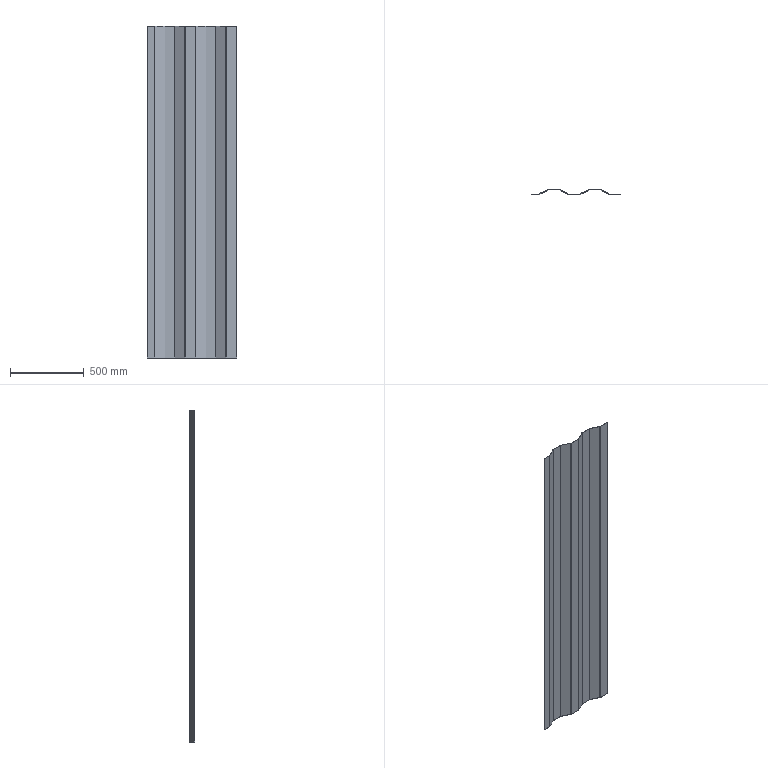Part | STEP file | 750078177 | 1 solid | 38 faces | box 606 x 36 x 2253 mm | volume 2873440 mm3 | plane 22 | cylinder 16 | commonest cylinder face diameters 6 x8 10 x8
STEP:
#1=CARTESIAN_POINT('',(116.472,35.472,0.));
#2=VERTEX_POINT('',#1);
#3=CARTESIAN_POINT('',(50.161,2.317,0.));
#4=VERTEX_POINT('',#3);
#5=CARTESIAN_POINT('',(117.106,35.789,0.));
#6=DIRECTION('',(-0.8944,-0.4472,0.));
#7=VECTOR('',#6,1000.);
#8=LINE('',#5,#7);
#9=EDGE_CURVE('',#2,#4,#8,.T.);
#10=ORIENTED_EDGE('',*,*,#9,.T.);
#11=CARTESIAN_POINT('',(50.161,2.317,2252.5));
#12=VERTEX_POINT('',#11);
#13=CARTESIAN_POINT('',(50.161,2.317,0.));
#14=DIRECTION('',(0.,0.,1.));
#15=VECTOR('',#14,1000.);
#16=LINE('',#13,#15);
#17=EDGE_CURVE('',#4,#12,#16,.T.);
#18=ORIENTED_EDGE('',*,*,#17,.T.);
#19=CARTESIAN_POINT('',(116.472,35.472,2252.5));
#20=VERTEX_POINT('',#19);
#21=CARTESIAN_POINT('',(117.106,35.789,2252.5));
#22=DIRECTION('',(0.8944,0.4472,0.));
#23=VECTOR('',#22,1000.);
#24=LINE('',#21,#23);
#25=EDGE_CURVE('',#12,#20,#24,.T.);
#26=ORIENTED_EDGE('',*,*,#25,.T.);
#27=CARTESIAN_POINT('',(116.472,35.472,0.));
#28=DIRECTION('',(0.,0.,-1.));
#29=VECTOR('',#28,1000.);
#30=LINE('',#27,#29);
#31=EDGE_CURVE('',#20,#2,#30,.T.);
#32=ORIENTED_EDGE('',*,*,#31,.T.);
#33=EDGE_LOOP('',(#10,#18,#26,#32));
#34=FACE_OUTER_BOUND('',#33,.T.);
#35=CARTESIAN_POINT('',(117.106,35.789,0.));
#36=DIRECTION('',(-0.4472,0.8944,0.));
#37=DIRECTION('',(-0.8944,-0.4472,0.));
#38=AXIS2_PLACEMENT_3D('',#35,#36,#37);
#39=PLANE('',#38);
#40=ADVANCED_FACE('',(#34),#39,.T.);
#41=ORIENTED_EDGE('',*,*,#17,.F.);
#42=CARTESIAN_POINT('',(48.82,2.,0.));
#43=VERTEX_POINT('',#42);
#44=CARTESIAN_POINT('',(48.82,5.,0.));
#45=DIRECTION('',(0.,0.,1.));
#46=DIRECTION('',(1.,0.,0.));
#47=AXIS2_PLACEMENT_3D('',#44,#45,#46);
#48=CIRCLE('',#47,3.);
#49=EDGE_CURVE('',#43,#4,#48,.T.);
#50=ORIENTED_EDGE('',*,*,#49,.F.);
#51=CARTESIAN_POINT('',(48.82,2.,2252.5));
#52=VERTEX_POINT('',#51);
#53=CARTESIAN_POINT('',(48.82,2.,0.));
#54=DIRECTION('',(0.,0.,-1.));
#55=VECTOR('',#54,1000.);
#56=LINE('',#53,#55);
#57=EDGE_CURVE('',#52,#43,#56,.T.);
#58=ORIENTED_EDGE('',*,*,#57,.F.);
#59=CARTESIAN_POINT('',(48.82,5.,2252.5));
#60=DIRECTION('',(0.,0.,-1.));
#61=DIRECTION('',(1.,0.,0.));
#62=AXIS2_PLACEMENT_3D('',#59,#60,#61);
#63=CIRCLE('',#62,3.);
#64=EDGE_CURVE('',#12,#52,#63,.T.);
#65=ORIENTED_EDGE('',*,*,#64,.F.);
#66=EDGE_LOOP('',(#41,#50,#58,#65));
#67=FACE_OUTER_BOUND('',#66,.T.);
#68=CARTESIAN_POINT('',(48.82,5.,0.));
#69=DIRECTION('',(0.,0.,1.));
#70=DIRECTION('',(1.,0.,0.));
#71=AXIS2_PLACEMENT_3D('',#68,#69,#70);
#72=CYLINDRICAL_SURFACE('',#71,3.);
#73=ADVANCED_FACE('',(#67),#72,.F.);
#74=CARTESIAN_POINT('',(535.18,2.,0.));
#75=VERTEX_POINT('',#74);
#76=CARTESIAN_POINT('',(606.,2.,0.));
#77=VERTEX_POINT('',#76);
#78=CARTESIAN_POINT('',(606.,2.,0.));
#79=DIRECTION('',(1.,0.,0.));
#80=VECTOR('',#79,1000.);
#81=LINE('',#78,#80);
#82=EDGE_CURVE('',#75,#77,#81,.T.);
#83=ORIENTED_EDGE('',*,*,#82,.T.);
#84=CARTESIAN_POINT('',(606.,0.,0.));
#85=VERTEX_POINT('',#84);
#86=CARTESIAN_POINT('',(606.,0.,0.));
#87=DIRECTION('',(0.,-1.,0.));
#88=VECTOR('',#87,1000.);
#89=LINE('',#86,#88);
#90=EDGE_CURVE('',#77,#85,#89,.T.);
#91=ORIENTED_EDGE('',*,*,#90,.T.);
#92=CARTESIAN_POINT('',(535.18,0.,0.));
#93=VERTEX_POINT('',#92);
#94=CARTESIAN_POINT('',(606.,0.,0.));
#95=DIRECTION('',(-1.,0.,0.));
#96=VECTOR('',#95,1000.);
#97=LINE('',#94,#96);
#98=EDGE_CURVE('',#85,#93,#97,.T.);
#99=ORIENTED_EDGE('',*,*,#98,.T.);
#100=CARTESIAN_POINT('',(532.944,0.5279,0.));
#101=VERTEX_POINT('',#100);
#102=CARTESIAN_POINT('',(535.18,5.,0.));
#103=DIRECTION('',(0.,0.,-1.));
#104=DIRECTION('',(1.,0.,0.));
#105=AXIS2_PLACEMENT_3D('',#102,#103,#104);
#106=CIRCLE('',#105,5.);
#107=EDGE_CURVE('',#93,#101,#106,.T.);
#108=ORIENTED_EDGE('',*,*,#107,.T.);
#109=CARTESIAN_POINT('',(466.633,33.683,0.));
#110=VERTEX_POINT('',#109);
#111=CARTESIAN_POINT('',(532.944,0.5279,0.));
#112=DIRECTION('',(-0.8944,0.4472,0.));
#113=VECTOR('',#112,1000.);
#114=LINE('',#111,#113);
#115=EDGE_CURVE('',#101,#110,#114,.T.);
#116=ORIENTED_EDGE('',*,*,#115,.T.);
#117=CARTESIAN_POINT('',(465.292,34.,0.));
#118=VERTEX_POINT('',#117);
#119=CARTESIAN_POINT('',(465.292,31.,0.));
#120=DIRECTION('',(0.,0.,1.));
#121=DIRECTION('',(1.,0.,0.));
#122=AXIS2_PLACEMENT_3D('',#119,#120,#121);
#123=CIRCLE('',#122,3.);
#124=EDGE_CURVE('',#110,#118,#123,.T.);
#125=ORIENTED_EDGE('',*,*,#124,.T.);
#126=CARTESIAN_POINT('',(396.708,34.,0.));
#127=VERTEX_POINT('',#126);
#128=CARTESIAN_POINT('',(606.,34.,0.));
#129=DIRECTION('',(-1.,0.,0.));
#130=VECTOR('',#129,1000.);
#131=LINE('',#128,#130);
#132=EDGE_CURVE('',#118,#127,#131,.T.);
#133=ORIENTED_EDGE('',*,*,#132,.T.);
#134=CARTESIAN_POINT('',(395.367,33.683,0.));
#135=VERTEX_POINT('',#134);
#136=CARTESIAN_POINT('',(396.708,31.,0.));
#137=DIRECTION('',(0.,0.,1.));
#138=DIRECTION('',(1.,0.,0.));
#139=AXIS2_PLACEMENT_3D('',#136,#137,#138);
#140=CIRCLE('',#139,3.);
#141=EDGE_CURVE('',#127,#135,#140,.T.);
#142=ORIENTED_EDGE('',*,*,#141,.T.);
#143=CARTESIAN_POINT('',(329.056,0.5279,0.));
#144=VERTEX_POINT('',#143);
#145=CARTESIAN_POINT('',(395.367,33.683,0.));
#146=DIRECTION('',(-0.8944,-0.4472,0.));
#147=VECTOR('',#146,1000.);
#148=LINE('',#145,#147);
#149=EDGE_CURVE('',#135,#144,#148,.T.);
#150=ORIENTED_EDGE('',*,*,#149,.T.);
#151=CARTESIAN_POINT('',(326.82,0.,0.));
#152=VERTEX_POINT('',#151);
#153=CARTESIAN_POINT('',(326.82,5.,0.));
#154=DIRECTION('',(0.,0.,-1.));
#155=DIRECTION('',(1.,0.,0.));
#156=AXIS2_PLACEMENT_3D('',#153,#154,#155);
#157=CIRCLE('',#156,5.);
#158=EDGE_CURVE('',#144,#152,#157,.T.);
#159=ORIENTED_EDGE('',*,*,#158,.T.);
#160=CARTESIAN_POINT('',(257.18,0.,0.));
#161=VERTEX_POINT('',#160);
#162=CARTESIAN_POINT('',(606.,0.,0.));
#163=DIRECTION('',(-1.,0.,0.));
#164=VECTOR('',#163,1000.);
#165=LINE('',#162,#164);
#166=EDGE_CURVE('',#152,#161,#165,.T.);
#167=ORIENTED_EDGE('',*,*,#166,.T.);
#168=CARTESIAN_POINT('',(254.944,0.5279,0.));
#169=VERTEX_POINT('',#168);
#170=CARTESIAN_POINT('',(257.18,5.,0.));
#171=DIRECTION('',(0.,0.,-1.));
#172=DIRECTION('',(1.,0.,0.));
#173=AXIS2_PLACEMENT_3D('',#170,#171,#172);
#174=CIRCLE('',#173,5.);
#175=EDGE_CURVE('',#161,#169,#174,.T.);
#176=ORIENTED_EDGE('',*,*,#175,.T.);
#177=CARTESIAN_POINT('',(188.633,33.683,0.));
#178=VERTEX_POINT('',#177);
#179=CARTESIAN_POINT('',(254.944,0.5279,0.));
#180=DIRECTION('',(-0.8944,0.4472,0.));
#181=VECTOR('',#180,1000.);
#182=LINE('',#179,#181);
#183=EDGE_CURVE('',#169,#178,#182,.T.);
#184=ORIENTED_EDGE('',*,*,#183,.T.);
#185=CARTESIAN_POINT('',(187.292,34.,0.));
#186=VERTEX_POINT('',#185);
#187=CARTESIAN_POINT('',(187.292,31.,0.));
#188=DIRECTION('',(0.,0.,1.));
#189=DIRECTION('',(1.,0.,0.));
#190=AXIS2_PLACEMENT_3D('',#187,#188,#189);
#191=CIRCLE('',#190,3.);
#192=EDGE_CURVE('',#178,#186,#191,.T.);
#193=ORIENTED_EDGE('',*,*,#192,.T.);
#194=CARTESIAN_POINT('',(118.708,34.,0.));
#195=VERTEX_POINT('',#194);
#196=CARTESIAN_POINT('',(606.,34.,0.));
#197=DIRECTION('',(-1.,0.,0.));
#198=VECTOR('',#197,1000.);
#199=LINE('',#196,#198);
#200=EDGE_CURVE('',#186,#195,#199,.T.);
#201=ORIENTED_EDGE('',*,*,#200,.T.);
#202=CARTESIAN_POINT('',(117.367,33.683,0.));
#203=VERTEX_POINT('',#202);
#204=CARTESIAN_POINT('',(118.708,31.,0.));
#205=DIRECTION('',(0.,0.,1.));
#206=DIRECTION('',(1.,0.,0.));
#207=AXIS2_PLACEMENT_3D('',#204,#205,#206);
#208=CIRCLE('',#207,3.);
#209=EDGE_CURVE('',#195,#203,#208,.T.);
#210=ORIENTED_EDGE('',*,*,#209,.T.);
#211=CARTESIAN_POINT('',(51.056,0.5279,0.));
#212=VERTEX_POINT('',#211);
#213=CARTESIAN_POINT('',(117.367,33.683,0.));
#214=DIRECTION('',(-0.8944,-0.4472,0.));
#215=VECTOR('',#214,1000.);
#216=LINE('',#213,#215);
#217=EDGE_CURVE('',#203,#212,#216,.T.);
#218=ORIENTED_EDGE('',*,*,#217,.T.);
#219=CARTESIAN_POINT('',(48.82,0.,0.));
#220=VERTEX_POINT('',#219);
#221=CARTESIAN_POINT('',(48.82,5.,0.));
#222=DIRECTION('',(0.,0.,-1.));
#223=DIRECTION('',(1.,0.,0.));
#224=AXIS2_PLACEMENT_3D('',#221,#222,#223);
#225=CIRCLE('',#224,5.);
#226=EDGE_CURVE('',#212,#220,#225,.T.);
#227=ORIENTED_EDGE('',*,*,#226,.T.);
#228=CARTESIAN_POINT('',(0.,0.,0.));
#229=VERTEX_POINT('',#228);
#230=CARTESIAN_POINT('',(606.,0.,0.));
#231=DIRECTION('',(-1.,0.,0.));
#232=VECTOR('',#231,1000.);
#233=LINE('',#230,#232);
#234=EDGE_CURVE('',#220,#229,#233,.T.);
#235=ORIENTED_EDGE('',*,*,#234,.T.);
#236=CARTESIAN_POINT('',(0.,2.,0.));
#237=VERTEX_POINT('',#236);
#238=CARTESIAN_POINT('',(0.,0.,0.));
#239=DIRECTION('',(0.,1.,0.));
#240=VECTOR('',#239,1000.);
#241=LINE('',#238,#240);
#242=EDGE_CURVE('',#229,#237,#241,.T.);
#243=ORIENTED_EDGE('',*,*,#242,.T.);
#244=CARTESIAN_POINT('',(606.,2.,0.));
#245=DIRECTION('',(1.,0.,0.));
#246=VECTOR('',#245,1000.);
#247=LINE('',#244,#246);
#248=EDGE_CURVE('',#237,#43,#247,.T.);
#249=ORIENTED_EDGE('',*,*,#248,.T.);
#250=ORIENTED_EDGE('',*,*,#49,.T.);
#251=ORIENTED_EDGE('',*,*,#9,.F.);
#252=CARTESIAN_POINT('',(118.708,36.,0.));
#253=VERTEX_POINT('',#252);
#254=CARTESIAN_POINT('',(118.708,31.,0.));
#255=DIRECTION('',(0.,0.,-1.));
#256=DIRECTION('',(1.,0.,0.));
#257=AXIS2_PLACEMENT_3D('',#254,#255,#256);
#258=CIRCLE('',#257,5.);
#259=EDGE_CURVE('',#2,#253,#258,.T.);
#260=ORIENTED_EDGE('',*,*,#259,.T.);
#261=CARTESIAN_POINT('',(187.292,36.,0.));
#262=VERTEX_POINT('',#261);
#263=CARTESIAN_POINT('',(606.,36.,0.));
#264=DIRECTION('',(1.,0.,0.));
#265=VECTOR('',#264,1000.);
#266=LINE('',#263,#265);
#267=EDGE_CURVE('',#253,#262,#266,.T.);
#268=ORIENTED_EDGE('',*,*,#267,.T.);
#269=CARTESIAN_POINT('',(189.528,35.472,0.));
#270=VERTEX_POINT('',#269);
#271=CARTESIAN_POINT('',(187.292,31.,0.));
#272=DIRECTION('',(0.,0.,-1.));
#273=DIRECTION('',(1.,0.,0.));
#274=AXIS2_PLACEMENT_3D('',#271,#272,#273);
#275=CIRCLE('',#274,5.);
#276=EDGE_CURVE('',#262,#270,#275,.T.);
#277=ORIENTED_EDGE('',*,*,#276,.T.);
#278=CARTESIAN_POINT('',(255.839,2.317,0.));
#279=VERTEX_POINT('',#278);
#280=CARTESIAN_POINT('',(189.528,35.472,0.));
#281=DIRECTION('',(0.8944,-0.4472,0.));
#282=VECTOR('',#281,1000.);
#283=LINE('',#280,#282);
#284=EDGE_CURVE('',#270,#279,#283,.T.);
#285=ORIENTED_EDGE('',*,*,#284,.T.);
#286=CARTESIAN_POINT('',(257.18,2.,0.));
#287=VERTEX_POINT('',#286);
#288=CARTESIAN_POINT('',(257.18,5.,0.));
#289=DIRECTION('',(0.,0.,1.));
#290=DIRECTION('',(1.,0.,0.));
#291=AXIS2_PLACEMENT_3D('',#288,#289,#290);
#292=CIRCLE('',#291,3.);
#293=EDGE_CURVE('',#279,#287,#292,.T.);
#294=ORIENTED_EDGE('',*,*,#293,.T.);
#295=CARTESIAN_POINT('',(326.82,2.,0.));
#296=VERTEX_POINT('',#295);
#297=CARTESIAN_POINT('',(606.,2.,0.));
#298=DIRECTION('',(1.,0.,0.));
#299=VECTOR('',#298,1000.);
#300=LINE('',#297,#299);
#301=EDGE_CURVE('',#287,#296,#300,.T.);
#302=ORIENTED_EDGE('',*,*,#301,.T.);
#303=CARTESIAN_POINT('',(328.161,2.317,0.));
#304=VERTEX_POINT('',#303);
#305=CARTESIAN_POINT('',(326.82,5.,0.));
#306=DIRECTION('',(0.,0.,1.));
#307=DIRECTION('',(1.,0.,0.));
#308=AXIS2_PLACEMENT_3D('',#305,#306,#307);
#309=CIRCLE('',#308,3.);
#310=EDGE_CURVE('',#296,#304,#309,.T.);
#311=ORIENTED_EDGE('',*,*,#310,.T.);
#312=CARTESIAN_POINT('',(394.472,35.472,0.));
#313=VERTEX_POINT('',#312);
#314=CARTESIAN_POINT('',(328.161,2.317,0.));
#315=DIRECTION('',(0.8944,0.4472,0.));
#316=VECTOR('',#315,1000.);
#317=LINE('',#314,#316);
#318=EDGE_CURVE('',#304,#313,#317,.T.);
#319=ORIENTED_EDGE('',*,*,#318,.T.);
#320=CARTESIAN_POINT('',(396.708,36.,0.));
#321=VERTEX_POINT('',#320);
#322=CARTESIAN_POINT('',(396.708,31.,0.));
#323=DIRECTION('',(0.,0.,-1.));
#324=DIRECTION('',(1.,0.,0.));
#325=AXIS2_PLACEMENT_3D('',#322,#323,#324);
#326=CIRCLE('',#325,5.);
#327=EDGE_CURVE('',#313,#321,#326,.T.);
#328=ORIENTED_EDGE('',*,*,#327,.T.);
#329=CARTESIAN_POINT('',(465.292,36.,0.));
#330=VERTEX_POINT('',#329);
#331=CARTESIAN_POINT('',(606.,36.,0.));
#332=DIRECTION('',(1.,0.,0.));
#333=VECTOR('',#332,1000.);
#334=LINE('',#331,#333);
#335=EDGE_CURVE('',#321,#330,#334,.T.);
#336=ORIENTED_EDGE('',*,*,#335,.T.);
#337=CARTESIAN_POINT('',(467.528,35.472,0.));
#338=VERTEX_POINT('',#337);
#339=CARTESIAN_POINT('',(465.292,31.,0.));
#340=DIRECTION('',(0.,0.,-1.));
#341=DIRECTION('',(1.,0.,0.));
#342=AXIS2_PLACEMENT_3D('',#339,#340,#341);
#343=CIRCLE('',#342,5.);
#344=EDGE_CURVE('',#330,#338,#343,.T.);
#345=ORIENTED_EDGE('',*,*,#344,.T.);
#346=CARTESIAN_POINT('',(533.839,2.317,0.));
#347=VERTEX_POINT('',#346);
#348=CARTESIAN_POINT('',(467.528,35.472,0.));
#349=DIRECTION('',(0.8944,-0.4472,0.));
#350=VECTOR('',#349,1000.);
#351=LINE('',#348,#350);
#352=EDGE_CURVE('',#338,#347,#351,.T.);
#353=ORIENTED_EDGE('',*,*,#352,.T.);
#354=CARTESIAN_POINT('',(535.18,5.,0.));
#355=DIRECTION('',(0.,0.,1.));
#356=DIRECTION('',(1.,0.,0.));
#357=AXIS2_PLACEMENT_3D('',#354,#355,#356);
#358=CIRCLE('',#357,3.);
#359=EDGE_CURVE('',#347,#75,#358,.T.);
#360=ORIENTED_EDGE('',*,*,#359,.T.);
#361=EDGE_LOOP('',(#83,#91,#99,#108,#116,#125,#133,#142,#150,#159,#167,#176,#184,#193,#201,#210,#218,#227,#235,#243,#249,#250,#251,#260,#268,#277,#285,#294,#302,#311,#319,#328,#336,#345,#353,#360));
#362=FACE_OUTER_BOUND('',#361,.T.);
#363=CARTESIAN_POINT('',(606.,0.,0.));
#364=DIRECTION('',(0.,0.,-1.));
#365=DIRECTION('',(-1.,0.,0.));
#366=AXIS2_PLACEMENT_3D('',#363,#364,#365);
#367=PLANE('',#366);
#368=ADVANCED_FACE('',(#362),#367,.T.);
#369=ORIENTED_EDGE('',*,*,#259,.F.);
#370=ORIENTED_EDGE('',*,*,#31,.F.);
#371=CARTESIAN_POINT('',(118.708,36.,2252.5));
#372=VERTEX_POINT('',#371);
#373=CARTESIAN_POINT('',(118.708,31.,2252.5));
#374=DIRECTION('',(0.,0.,-1.));
#375=DIRECTION('',(1.,0.,0.));
#376=AXIS2_PLACEMENT_3D('',#373,#374,#375);
#377=CIRCLE('',#376,5.);
#378=EDGE_CURVE('',#20,#372,#377,.T.);
#379=ORIENTED_EDGE('',*,*,#378,.T.);
#380=CARTESIAN_POINT('',(118.708,36.,0.));
#381=DIRECTION('',(0.,0.,-1.));
#382=VECTOR('',#381,1000.);
#383=LINE('',#380,#382);
#384=EDGE_CURVE('',#372,#253,#383,.T.);
#385=ORIENTED_EDGE('',*,*,#384,.T.);
#386=EDGE_LOOP('',(#369,#370,#379,#385));
#387=FACE_OUTER_BOUND('',#386,.T.);
#388=CARTESIAN_POINT('',(118.708,31.,0.));
#389=DIRECTION('',(0.,0.,1.));
#390=DIRECTION('',(1.,0.,0.));
#391=AXIS2_PLACEMENT_3D('',#388,#389,#390);
#392=CYLINDRICAL_SURFACE('',#391,5.);
#393=ADVANCED_FACE('',(#387),#392,.T.);
#394=CARTESIAN_POINT('',(467.528,35.472,2252.5));
#395=VERTEX_POINT('',#394);
#396=CARTESIAN_POINT('',(533.839,2.317,2252.5));
#397=VERTEX_POINT('',#396);
#398=CARTESIAN_POINT('',(467.528,35.472,2252.5));
#399=DIRECTION('',(0.8944,-0.4472,0.));
#400=VECTOR('',#399,1000.);
#401=LINE('',#398,#400);
#402=EDGE_CURVE('',#395,#397,#401,.T.);
#403=ORIENTED_EDGE('',*,*,#402,.F.);
#404=CARTESIAN_POINT('',(465.292,36.,2252.5));
#405=VERTEX_POINT('',#404);
#406=CARTESIAN_POINT('',(465.292,31.,2252.5));
#407=DIRECTION('',(0.,0.,-1.));
#408=DIRECTION('',(1.,0.,0.));
#409=AXIS2_PLACEMENT_3D('',#406,#407,#408);
#410=CIRCLE('',#409,5.);
#411=EDGE_CURVE('',#405,#395,#410,.T.);
#412=ORIENTED_EDGE('',*,*,#411,.F.);
#413=CARTESIAN_POINT('',(396.708,36.,2252.5));
#414=VERTEX_POINT('',#413);
#415=CARTESIAN_POINT('',(535.18,36.,2252.5));
#416=DIRECTION('',(1.,0.,0.));
#417=VECTOR('',#416,1000.);
#418=LINE('',#415,#417);
#419=EDGE_CURVE('',#414,#405,#418,.T.);
#420=ORIENTED_EDGE('',*,*,#419,.F.);
#421=CARTESIAN_POINT('',(394.472,35.472,2252.5));
#422=VERTEX_POINT('',#421);
#423=CARTESIAN_POINT('',(396.708,31.,2252.5));
#424=DIRECTION('',(0.,0.,-1.));
#425=DIRECTION('',(1.,0.,0.));
#426=AXIS2_PLACEMENT_3D('',#423,#424,#425);
#427=CIRCLE('',#426,5.);
#428=EDGE_CURVE('',#422,#414,#427,.T.);
#429=ORIENTED_EDGE('',*,*,#428,.F.);
#430=CARTESIAN_POINT('',(328.161,2.317,2252.5));
#431=VERTEX_POINT('',#430);
#432=CARTESIAN_POINT('',(328.161,2.317,2252.5));
#433=DIRECTION('',(0.8944,0.4472,0.));
#434=VECTOR('',#433,1000.);
#435=LINE('',#432,#434);
#436=EDGE_CURVE('',#431,#422,#435,.T.);
#437=ORIENTED_EDGE('',*,*,#436,.F.);
#438=CARTESIAN_POINT('',(326.82,2.,2252.5));
#439=VERTEX_POINT('',#438);
#440=CARTESIAN_POINT('',(326.82,5.,2252.5));
#441=DIRECTION('',(0.,0.,-1.));
#442=DIRECTION('',(1.,0.,0.));
#443=AXIS2_PLACEMENT_3D('',#440,#441,#442);
#444=CIRCLE('',#443,3.);
#445=EDGE_CURVE('',#431,#439,#444,.T.);
#446=ORIENTED_EDGE('',*,*,#445,.T.);
#447=CARTESIAN_POINT('',(257.18,2.,2252.5));
#448=VERTEX_POINT('',#447);
#449=CARTESIAN_POINT('',(535.18,2.,2252.5));
#450=DIRECTION('',(1.,0.,0.));
#451=VECTOR('',#450,1000.);
#452=LINE('',#449,#451);
#453=EDGE_CURVE('',#448,#439,#452,.T.);
#454=ORIENTED_EDGE('',*,*,#453,.F.);
#455=CARTESIAN_POINT('',(255.839,2.317,2252.5));
#456=VERTEX_POINT('',#455);
#457=CARTESIAN_POINT('',(257.18,5.,2252.5));
#458=DIRECTION('',(0.,0.,-1.));
#459=DIRECTION('',(1.,0.,0.));
#460=AXIS2_PLACEMENT_3D('',#457,#458,#459);
#461=CIRCLE('',#460,3.);
#462=EDGE_CURVE('',#448,#456,#461,.T.);
#463=ORIENTED_EDGE('',*,*,#462,.T.);
#464=CARTESIAN_POINT('',(189.528,35.472,2252.5));
#465=VERTEX_POINT('',#464);
#466=CARTESIAN_POINT('',(189.528,35.472,2252.5));
#467=DIRECTION('',(0.8944,-0.4472,0.));
#468=VECTOR('',#467,1000.);
#469=LINE('',#466,#468);
#470=EDGE_CURVE('',#465,#456,#469,.T.);
#471=ORIENTED_EDGE('',*,*,#470,.F.);
#472=CARTESIAN_POINT('',(187.292,36.,2252.5));
#473=VERTEX_POINT('',#472);
#474=CARTESIAN_POINT('',(187.292,31.,2252.5));
#475=DIRECTION('',(0.,0.,-1.));
#476=DIRECTION('',(1.,0.,0.));
#477=AXIS2_PLACEMENT_3D('',#474,#475,#476);
#478=CIRCLE('',#477,5.);
#479=EDGE_CURVE('',#473,#465,#478,.T.);
#480=ORIENTED_EDGE('',*,*,#479,.F.);
#481=CARTESIAN_POINT('',(535.18,36.,2252.5));
#482=DIRECTION('',(1.,0.,0.));
#483=VECTOR('',#482,1000.);
#484=LINE('',#481,#483);
#485=EDGE_CURVE('',#372,#473,#484,.T.);
#486=ORIENTED_EDGE('',*,*,#485,.F.);
#487=ORIENTED_EDGE('',*,*,#378,.F.);
#488=ORIENTED_EDGE('',*,*,#25,.F.);
#489=ORIENTED_EDGE('',*,*,#64,.T.);
#490=CARTESIAN_POINT('',(0.,2.,2252.5));
#491=VERTEX_POINT('',#490);
#492=CARTESIAN_POINT('',(535.18,2.,2252.5));
#493=DIRECTION('',(1.,0.,0.));
#494=VECTOR('',#493,1000.);
#495=LINE('',#492,#494);
#496=EDGE_CURVE('',#491,#52,#495,.T.);
#497=ORIENTED_EDGE('',*,*,#496,.F.);
#498=CARTESIAN_POINT('',(0.,0.,2252.5));
#499=VERTEX_POINT('',#498);
#500=CARTESIAN_POINT('',(0.,5.,2252.5));
#501=DIRECTION('',(0.,1.,0.));
#502=VECTOR('',#501,1000.);
#503=LINE('',#500,#502);
#504=EDGE_CURVE('',#499,#491,#503,.T.);
#505=ORIENTED_EDGE('',*,*,#504,.F.);
#506=CARTESIAN_POINT('',(48.82,0.,2252.5));
#507=VERTEX_POINT('',#506);
#508=CARTESIAN_POINT('',(535.18,0.,2252.5));
#509=DIRECTION('',(-1.,0.,0.));
#510=VECTOR('',#509,1000.);
#511=LINE('',#508,#510);
#512=EDGE_CURVE('',#507,#499,#511,.T.);
#513=ORIENTED_EDGE('',*,*,#512,.F.);
#514=CARTESIAN_POINT('',(51.056,0.5279,2252.5));
#515=VERTEX_POINT('',#514);
#516=CARTESIAN_POINT('',(48.82,5.,2252.5));
#517=DIRECTION('',(0.,0.,-1.));
#518=DIRECTION('',(1.,0.,0.));
#519=AXIS2_PLACEMENT_3D('',#516,#517,#518);
#520=CIRCLE('',#519,5.);
#521=EDGE_CURVE('',#515,#507,#520,.T.);
#522=ORIENTED_EDGE('',*,*,#521,.F.);
#523=CARTESIAN_POINT('',(117.367,33.683,2252.5));
#524=VERTEX_POINT('',#523);
#525=CARTESIAN_POINT('',(117.367,33.683,2252.5));
#526=DIRECTION('',(-0.8944,-0.4472,0.));
#527=VECTOR('',#526,1000.);
#528=LINE('',#525,#527);
#529=EDGE_CURVE('',#524,#515,#528,.T.);
#530=ORIENTED_EDGE('',*,*,#529,.F.);
#531=CARTESIAN_POINT('',(118.708,34.,2252.5));
#532=VERTEX_POINT('',#531);
#533=CARTESIAN_POINT('',(118.708,31.,2252.5));
#534=DIRECTION('',(0.,0.,-1.));
#535=DIRECTION('',(1.,0.,0.));
#536=AXIS2_PLACEMENT_3D('',#533,#534,#535);
#537=CIRCLE('',#536,3.);
#538=EDGE_CURVE('',#524,#532,#537,.T.);
#539=ORIENTED_EDGE('',*,*,#538,.T.);
#540=CARTESIAN_POINT('',(187.292,34.,2252.5));
#541=VERTEX_POINT('',#540);
#542=CARTESIAN_POINT('',(535.18,34.,2252.5));
#543=DIRECTION('',(-1.,0.,0.));
#544=VECTOR('',#543,1000.);
#545=LINE('',#542,#544);
#546=EDGE_CURVE('',#541,#532,#545,.T.);
#547=ORIENTED_EDGE('',*,*,#546,.F.);
#548=CARTESIAN_POINT('',(188.633,33.683,2252.5));
#549=VERTEX_POINT('',#548);
#550=CARTESIAN_POINT('',(187.292,31.,2252.5));
#551=DIRECTION('',(0.,0.,-1.));
#552=DIRECTION('',(1.,0.,0.));
#553=AXIS2_PLACEMENT_3D('',#550,#551,#552);
#554=CIRCLE('',#553,3.);
#555=EDGE_CURVE('',#541,#549,#554,.T.);
#556=ORIENTED_EDGE('',*,*,#555,.T.);
#557=CARTESIAN_POINT('',(254.944,0.5279,2252.5));
#558=VERTEX_POINT('',#557);
#559=CARTESIAN_POINT('',(254.944,0.5279,2252.5));
#560=DIRECTION('',(-0.8944,0.4472,0.));
#561=VECTOR('',#560,1000.);
#562=LINE('',#559,#561);
#563=EDGE_CURVE('',#558,#549,#562,.T.);
#564=ORIENTED_EDGE('',*,*,#563,.F.);
#565=CARTESIAN_POINT('',(257.18,0.,2252.5));
#566=VERTEX_POINT('',#565);
#567=CARTESIAN_POINT('',(257.18,5.,2252.5));
#568=DIRECTION('',(0.,0.,-1.));
#569=DIRECTION('',(1.,0.,0.));
#570=AXIS2_PLACEMENT_3D('',#567,#568,#569);
#571=CIRCLE('',#570,5.);
#572=EDGE_CURVE('',#566,#558,#571,.T.);
#573=ORIENTED_EDGE('',*,*,#572,.F.);
#574=CARTESIAN_POINT('',(326.82,0.,2252.5));
#575=VERTEX_POINT('',#574);
#576=CARTESIAN_POINT('',(535.18,0.,2252.5));
#577=DIRECTION('',(-1.,0.,0.));
#578=VECTOR('',#577,1000.);
#579=LINE('',#576,#578);
#580=EDGE_CURVE('',#575,#566,#579,.T.);
#581=ORIENTED_EDGE('',*,*,#580,.F.);
#582=CARTESIAN_POINT('',(329.056,0.5279,2252.5));
#583=VERTEX_POINT('',#582);
#584=CARTESIAN_POINT('',(326.82,5.,2252.5));
#585=DIRECTION('',(0.,0.,-1.));
#586=DIRECTION('',(1.,0.,0.));
#587=AXIS2_PLACEMENT_3D('',#584,#585,#586);
#588=CIRCLE('',#587,5.);
#589=EDGE_CURVE('',#583,#575,#588,.T.);
#590=ORIENTED_EDGE('',*,*,#589,.F.);
#591=CARTESIAN_POINT('',(395.367,33.683,2252.5));
#592=VERTEX_POINT('',#591);
#593=CARTESIAN_POINT('',(395.367,33.683,2252.5));
#594=DIRECTION('',(-0.8944,-0.4472,0.));
#595=VECTOR('',#594,1000.);
#596=LINE('',#593,#595);
#597=EDGE_CURVE('',#592,#583,#596,.T.);
#598=ORIENTED_EDGE('',*,*,#597,.F.);
#599=CARTESIAN_POINT('',(396.708,34.,2252.5));
#600=VERTEX_POINT('',#599);
#601=CARTESIAN_POINT('',(396.708,31.,2252.5));
#602=DIRECTION('',(0.,0.,-1.));
#603=DIRECTION('',(1.,0.,0.));
#604=AXIS2_PLACEMENT_3D('',#601,#602,#603);
#605=CIRCLE('',#604,3.);
#606=EDGE_CURVE('',#592,#600,#605,.T.);
#607=ORIENTED_EDGE('',*,*,#606,.T.);
#608=CARTESIAN_POINT('',(465.292,34.,2252.5));
#609=VERTEX_POINT('',#608);
#610=CARTESIAN_POINT('',(535.18,34.,2252.5));
#611=DIRECTION('',(-1.,0.,0.));
#612=VECTOR('',#611,1000.);
#613=LINE('',#610,#612);
#614=EDGE_CURVE('',#609,#600,#613,.T.);
#615=ORIENTED_EDGE('',*,*,#614,.F.);
#616=CARTESIAN_POINT('',(466.633,33.683,2252.5));
#617=VERTEX_POINT('',#616);
#618=CARTESIAN_POINT('',(465.292,31.,2252.5));
#619=DIRECTION('',(0.,0.,-1.));
#620=DIRECTION('',(1.,0.,0.));
#621=AXIS2_PLACEMENT_3D('',#618,#619,#620);
#622=CIRCLE('',#621,3.);
#623=EDGE_CURVE('',#609,#617,#622,.T.);
#624=ORIENTED_EDGE('',*,*,#623,.T.);
#625=CARTESIAN_POINT('',(532.944,0.5279,2252.5));
#626=VERTEX_POINT('',#625);
#627=CARTESIAN_POINT('',(532.944,0.5279,2252.5));
#628=DIRECTION('',(-0.8944,0.4472,0.));
#629=VECTOR('',#628,1000.);
#630=LINE('',#627,#629);
#631=EDGE_CURVE('',#626,#617,#630,.T.);
#632=ORIENTED_EDGE('',*,*,#631,.F.);
#633=CARTESIAN_POINT('',(535.18,0.,2252.5));
#634=VERTEX_POINT('',#633);
#635=CARTESIAN_POINT('',(535.18,5.,2252.5));
#636=DIRECTION('',(0.,0.,-1.));
#637=DIRECTION('',(1.,0.,0.));
#638=AXIS2_PLACEMENT_3D('',#635,#636,#637);
#639=CIRCLE('',#638,5.);
#640=EDGE_CURVE('',#634,#626,#639,.T.);
#641=ORIENTED_EDGE('',*,*,#640,.F.);
#642=CARTESIAN_POINT('',(606.,0.,2252.5));
#643=VERTEX_POINT('',#642);
#644=CARTESIAN_POINT('',(535.18,0.,2252.5));
#645=DIRECTION('',(-1.,0.,0.));
#646=VECTOR('',#645,1000.);
#647=LINE('',#644,#646);
#648=EDGE_CURVE('',#643,#634,#647,.T.);
#649=ORIENTED_EDGE('',*,*,#648,.F.);
#650=CARTESIAN_POINT('',(606.,2.,2252.5));
#651=VERTEX_POINT('',#650);
#652=CARTESIAN_POINT('',(606.,5.,2252.5));
#653=DIRECTION('',(0.,-1.,0.));
#654=VECTOR('',#653,1000.);
#655=LINE('',#652,#654);
#656=EDGE_CURVE('',#651,#643,#655,.T.);
#657=ORIENTED_EDGE('',*,*,#656,.F.);
#658=CARTESIAN_POINT('',(535.18,2.,2252.5));
#659=VERTEX_POINT('',#658);
#660=CARTESIAN_POINT('',(535.18,2.,2252.5));
#661=DIRECTION('',(1.,0.,0.));
#662=VECTOR('',#661,1000.);
#663=LINE('',#660,#662);
#664=EDGE_CURVE('',#659,#651,#663,.T.);
#665=ORIENTED_EDGE('',*,*,#664,.F.);
#666=CARTESIAN_POINT('',(535.18,5.,2252.5));
#667=DIRECTION('',(0.,0.,-1.));
#668=DIRECTION('',(1.,0.,0.));
#669=AXIS2_PLACEMENT_3D('',#666,#667,#668);
#670=CIRCLE('',#669,3.);
#671=EDGE_CURVE('',#659,#397,#670,.T.);
#672=ORIENTED_EDGE('',*,*,#671,.T.);
#673=EDGE_LOOP('',(#403,#412,#420,#429,#437,#446,#454,#463,#471,#480,#486,#487,#488,#489,#497,#505,#513,#522,#530,#539,#547,#556,#564,#573,#581,#590,#598,#607,#615,#624,#632,#641,#649,#657,#665,#672));
#674=FACE_OUTER_BOUND('',#673,.T.);
#675=CARTESIAN_POINT('',(535.18,5.,2252.5));
#676=DIRECTION('',(0.,0.,-1.));
#677=DIRECTION('',(-1.,0.,0.));
#678=AXIS2_PLACEMENT_3D('',#675,#676,#677);
#679=PLANE('',#678);
#680=ADVANCED_FACE('',(#674),#679,.F.);
#681=ORIENTED_EDGE('',*,*,#248,.F.);
#682=CARTESIAN_POINT('',(0.,2.,0.));
#683=DIRECTION('',(0.,0.,1.));
#684=VECTOR('',#683,1000.);
#685=LINE('',#682,#684);
#686=EDGE_CURVE('',#237,#491,#685,.T.);
#687=ORIENTED_EDGE('',*,*,#686,.T.);
#688=ORIENTED_EDGE('',*,*,#496,.T.);
#689=ORIENTED_EDGE('',*,*,#57,.T.);
#690=EDGE_LOOP('',(#681,#687,#688,#689));
#691=FACE_OUTER_BOUND('',#690,.T.);
#692=CARTESIAN_POINT('',(50.,2.,0.));
#693=DIRECTION('',(0.,1.,0.));
#694=DIRECTION('',(-1.,0.,0.));
#695=AXIS2_PLACEMENT_3D('',#692,#693,#694);
#696=PLANE('',#695);
#697=ADVANCED_FACE('',(#691),#696,.T.);
#698=CARTESIAN_POINT('',(606.,2.,0.));
#699=DIRECTION('',(0.,0.,-1.));
#700=VECTOR('',#699,1000.);
#701=LINE('',#698,#700);
#702=EDGE_CURVE('',#651,#77,#701,.T.);
#703=ORIENTED_EDGE('',*,*,#702,.F.);
#704=ORIENTED_EDGE('',*,*,#656,.T.);
#705=CARTESIAN_POINT('',(606.,0.,0.));
#706=DIRECTION('',(0.,0.,1.));
#707=VECTOR('',#706,1000.);
#708=LINE('',#705,#707);
#709=EDGE_CURVE('',#85,#643,#708,.T.);
#710=ORIENTED_EDGE('',*,*,#709,.F.);
#711=ORIENTED_EDGE('',*,*,#90,.F.);
#712=EDGE_LOOP('',(#703,#704,#710,#711));
#713=FACE_OUTER_BOUND('',#712,.T.);
#714=CARTESIAN_POINT('',(606.,0.,0.));
#715=DIRECTION('',(-1.,0.,0.));
#716=DIRECTION('',(0.,-1.,0.));
#717=AXIS2_PLACEMENT_3D('',#714,#715,#716);
#718=PLANE('',#717);
#719=ADVANCED_FACE('',(#713),#718,.F.);
#720=ORIENTED_EDGE('',*,*,#82,.F.);
#721=CARTESIAN_POINT('',(535.18,2.,0.));
#722=DIRECTION('',(0.,0.,1.));
#723=VECTOR('',#722,1000.);
#724=LINE('',#721,#723);
#725=EDGE_CURVE('',#75,#659,#724,.T.);
#726=ORIENTED_EDGE('',*,*,#725,.T.);
#727=ORIENTED_EDGE('',*,*,#664,.T.);
#728=ORIENTED_EDGE('',*,*,#702,.T.);
#729=EDGE_LOOP('',(#720,#726,#727,#728));
#730=FACE_OUTER_BOUND('',#729,.T.);
#731=CARTESIAN_POINT('',(606.,2.,0.));
#732=DIRECTION('',(0.,1.,0.));
#733=DIRECTION('',(-1.,0.,0.));
#734=AXIS2_PLACEMENT_3D('',#731,#732,#733);
#735=PLANE('',#734);
#736=ADVANCED_FACE('',(#730),#735,.T.);
#737=ORIENTED_EDGE('',*,*,#352,.F.);
#738=CARTESIAN_POINT('',(467.528,35.472,0.));
#739=DIRECTION('',(0.,0.,1.));
#740=VECTOR('',#739,1000.);
#741=LINE('',#738,#740);
#742=EDGE_CURVE('',#338,#395,#741,.T.);
#743=ORIENTED_EDGE('',*,*,#742,.T.);
#744=ORIENTED_EDGE('',*,*,#402,.T.);
#745=CARTESIAN_POINT('',(533.839,2.317,0.));
#746=DIRECTION('',(0.,0.,-1.));
#747=VECTOR('',#746,1000.);
#748=LINE('',#745,#747);
#749=EDGE_CURVE('',#397,#347,#748,.T.);
#750=ORIENTED_EDGE('',*,*,#749,.T.);
#751=EDGE_LOOP('',(#737,#743,#744,#750));
#752=FACE_OUTER_BOUND('',#751,.T.);
#753=CARTESIAN_POINT('',(534.894,1.789,0.));
#754=DIRECTION('',(0.4472,0.8944,0.));
#755=DIRECTION('',(-0.8944,0.4472,0.));
#756=AXIS2_PLACEMENT_3D('',#753,#754,#755);
#757=PLANE('',#756);
#758=ADVANCED_FACE('',(#752),#757,.T.);
#759=ORIENTED_EDGE('',*,*,#344,.F.);
#760=CARTESIAN_POINT('',(465.292,36.,0.));
#761=DIRECTION('',(0.,0.,1.));
#762=VECTOR('',#761,1000.);
#763=LINE('',#760,#762);
#764=EDGE_CURVE('',#330,#405,#763,.T.);
#765=ORIENTED_EDGE('',*,*,#764,.T.);
#766=ORIENTED_EDGE('',*,*,#411,.T.);
#767=ORIENTED_EDGE('',*,*,#742,.F.);
#768=EDGE_LOOP('',(#759,#765,#766,#767));
#769=FACE_OUTER_BOUND('',#768,.T.);
#770=CARTESIAN_POINT('',(465.292,31.,0.));
#771=DIRECTION('',(0.,0.,1.));
#772=DIRECTION('',(1.,0.,0.));
#773=AXIS2_PLACEMENT_3D('',#770,#771,#772);
#774=CYLINDRICAL_SURFACE('',#773,5.);
#775=ADVANCED_FACE('',(#769),#774,.T.);
#776=ORIENTED_EDGE('',*,*,#335,.F.);
#777=CARTESIAN_POINT('',(396.708,36.,0.));
#778=DIRECTION('',(0.,0.,1.));
#779=VECTOR('',#778,1000.);
#780=LINE('',#777,#779);
#781=EDGE_CURVE('',#321,#414,#780,.T.);
#782=ORIENTED_EDGE('',*,*,#781,.T.);
#783=ORIENTED_EDGE('',*,*,#419,.T.);
#784=ORIENTED_EDGE('',*,*,#764,.F.);
#785=EDGE_LOOP('',(#776,#782,#783,#784));
#786=FACE_OUTER_BOUND('',#785,.T.);
#787=CARTESIAN_POINT('',(466.,36.,0.));
#788=DIRECTION('',(0.,1.,0.));
#789=DIRECTION('',(-1.,0.,0.));
#790=AXIS2_PLACEMENT_3D('',#787,#788,#789);
#791=PLANE('',#790);
#792=ADVANCED_FACE('',(#786),#791,.T.);
#793=ORIENTED_EDGE('',*,*,#327,.F.);
#794=CARTESIAN_POINT('',(394.472,35.472,0.));
#795=DIRECTION('',(0.,0.,1.));
#796=VECTOR('',#795,1000.);
#797=LINE('',#794,#796);
#798=EDGE_CURVE('',#313,#422,#797,.T.);
#799=ORIENTED_EDGE('',*,*,#798,.T.);
#800=ORIENTED_EDGE('',*,*,#428,.T.);
#801=ORIENTED_EDGE('',*,*,#781,.F.);
#802=EDGE_LOOP('',(#793,#799,#800,#801));
#803=FACE_OUTER_BOUND('',#802,.T.);
#804=CARTESIAN_POINT('',(396.708,31.,0.));
#805=DIRECTION('',(0.,0.,1.));
#806=DIRECTION('',(1.,0.,0.));
#807=AXIS2_PLACEMENT_3D('',#804,#805,#806);
#808=CYLINDRICAL_SURFACE('',#807,5.);
#809=ADVANCED_FACE('',(#803),#808,.T.);
#810=ORIENTED_EDGE('',*,*,#318,.F.);
#811=CARTESIAN_POINT('',(328.161,2.317,0.));
#812=DIRECTION('',(0.,0.,1.));
#813=VECTOR('',#812,1000.);
#814=LINE('',#811,#813);
#815=EDGE_CURVE('',#304,#431,#814,.T.);
#816=ORIENTED_EDGE('',*,*,#815,.T.);
#817=ORIENTED_EDGE('',*,*,#436,.T.);
#818=ORIENTED_EDGE('',*,*,#798,.F.);
#819=EDGE_LOOP('',(#810,#816,#817,#818));
#820=FACE_OUTER_BOUND('',#819,.T.);
#821=CARTESIAN_POINT('',(395.106,35.789,0.));
#822=DIRECTION('',(-0.4472,0.8944,0.));
#823=DIRECTION('',(-0.8944,-0.4472,0.));
#824=AXIS2_PLACEMENT_3D('',#821,#822,#823);
#825=PLANE('',#824);
#826=ADVANCED_FACE('',(#820),#825,.T.);
#827=ORIENTED_EDGE('',*,*,#301,.F.);
#828=CARTESIAN_POINT('',(257.18,2.,0.));
#829=DIRECTION('',(0.,0.,1.));
#830=VECTOR('',#829,1000.);
#831=LINE('',#828,#830);
#832=EDGE_CURVE('',#287,#448,#831,.T.);
#833=ORIENTED_EDGE('',*,*,#832,.T.);
#834=ORIENTED_EDGE('',*,*,#453,.T.);
#835=CARTESIAN_POINT('',(326.82,2.,0.));
#836=DIRECTION('',(0.,0.,-1.));
#837=VECTOR('',#836,1000.);
#838=LINE('',#835,#837);
#839=EDGE_CURVE('',#439,#296,#838,.T.);
#840=ORIENTED_EDGE('',*,*,#839,.T.);
#841=EDGE_LOOP('',(#827,#833,#834,#840));
#842=FACE_OUTER_BOUND('',#841,.T.);
#843=CARTESIAN_POINT('',(328.,2.,0.));
#844=DIRECTION('',(0.,1.,0.));
#845=DIRECTION('',(-1.,0.,0.));
#846=AXIS2_PLACEMENT_3D('',#843,#844,#845);
#847=PLANE('',#846);
#848=ADVANCED_FACE('',(#842),#847,.T.);
#849=ORIENTED_EDGE('',*,*,#284,.F.);
#850=CARTESIAN_POINT('',(189.528,35.472,0.));
#851=DIRECTION('',(0.,0.,1.));
#852=VECTOR('',#851,1000.);
#853=LINE('',#850,#852);
#854=EDGE_CURVE('',#270,#465,#853,.T.);
#855=ORIENTED_EDGE('',*,*,#854,.T.);
#856=ORIENTED_EDGE('',*,*,#470,.T.);
#857=CARTESIAN_POINT('',(255.839,2.317,0.));
#858=DIRECTION('',(0.,0.,-1.));
#859=VECTOR('',#858,1000.);
#860=LINE('',#857,#859);
#861=EDGE_CURVE('',#456,#279,#860,.T.);
#862=ORIENTED_EDGE('',*,*,#861,.T.);
#863=EDGE_LOOP('',(#849,#855,#856,#862));
#864=FACE_OUTER_BOUND('',#863,.T.);
#865=CARTESIAN_POINT('',(256.894,1.789,0.));
#866=DIRECTION('',(0.4472,0.8944,0.));
#867=DIRECTION('',(-0.8944,0.4472,0.));
#868=AXIS2_PLACEMENT_3D('',#865,#866,#867);
#869=PLANE('',#868);
#870=ADVANCED_FACE('',(#864),#869,.T.);
#871=ORIENTED_EDGE('',*,*,#276,.F.);
#872=CARTESIAN_POINT('',(187.292,36.,0.));
#873=DIRECTION('',(0.,0.,1.));
#874=VECTOR('',#873,1000.);
#875=LINE('',#872,#874);
#876=EDGE_CURVE('',#262,#473,#875,.T.);
#877=ORIENTED_EDGE('',*,*,#876,.T.);
#878=ORIENTED_EDGE('',*,*,#479,.T.);
#879=ORIENTED_EDGE('',*,*,#854,.F.);
#880=EDGE_LOOP('',(#871,#877,#878,#879));
#881=FACE_OUTER_BOUND('',#880,.T.);
#882=CARTESIAN_POINT('',(187.292,31.,0.));
#883=DIRECTION('',(0.,0.,1.));
#884=DIRECTION('',(1.,0.,0.));
#885=AXIS2_PLACEMENT_3D('',#882,#883,#884);
#886=CYLINDRICAL_SURFACE('',#885,5.);
#887=ADVANCED_FACE('',(#881),#886,.T.);
#888=ORIENTED_EDGE('',*,*,#267,.F.);
#889=ORIENTED_EDGE('',*,*,#384,.F.);
#890=ORIENTED_EDGE('',*,*,#485,.T.);
#891=ORIENTED_EDGE('',*,*,#876,.F.);
#892=EDGE_LOOP('',(#888,#889,#890,#891));
#893=FACE_OUTER_BOUND('',#892,.T.);
#894=CARTESIAN_POINT('',(188.,36.,0.));
#895=DIRECTION('',(0.,1.,0.));
#896=DIRECTION('',(-1.,0.,0.));
#897=AXIS2_PLACEMENT_3D('',#894,#895,#896);
#898=PLANE('',#897);
#899=ADVANCED_FACE('',(#893),#898,.T.);
#900=ORIENTED_EDGE('',*,*,#242,.F.);
#901=CARTESIAN_POINT('',(0.,0.,0.));
#902=DIRECTION('',(0.,0.,1.));
#903=VECTOR('',#902,1000.);
#904=LINE('',#901,#903);
#905=EDGE_CURVE('',#229,#499,#904,.T.);
#906=ORIENTED_EDGE('',*,*,#905,.T.);
#907=ORIENTED_EDGE('',*,*,#504,.T.);
#908=ORIENTED_EDGE('',*,*,#686,.F.);
#909=EDGE_LOOP('',(#900,#906,#907,#908));
#910=FACE_OUTER_BOUND('',#909,.T.);
#911=CARTESIAN_POINT('',(0.,0.,0.));
#912=DIRECTION('',(-1.,0.,0.));
#913=DIRECTION('',(0.,-1.,0.));
#914=AXIS2_PLACEMENT_3D('',#911,#912,#913);
#915=PLANE('',#914);
#916=ADVANCED_FACE('',(#910),#915,.T.);
#917=ORIENTED_EDGE('',*,*,#905,.F.);
#918=ORIENTED_EDGE('',*,*,#234,.F.);
#919=CARTESIAN_POINT('',(48.82,0.,0.));
#920=DIRECTION('',(0.,0.,-1.));
#921=VECTOR('',#920,1000.);
#922=LINE('',#919,#921);
#923=EDGE_CURVE('',#507,#220,#922,.T.);
#924=ORIENTED_EDGE('',*,*,#923,.F.);
#925=ORIENTED_EDGE('',*,*,#512,.T.);
#926=EDGE_LOOP('',(#917,#918,#924,#925));
#927=FACE_OUTER_BOUND('',#926,.T.);
#928=CARTESIAN_POINT('',(50.,0.,0.));
#929=DIRECTION('',(0.,1.,0.));
#930=DIRECTION('',(-1.,0.,0.));
#931=AXIS2_PLACEMENT_3D('',#928,#929,#930);
#932=PLANE('',#931);
#933=ADVANCED_FACE('',(#927),#932,.F.);
#934=ORIENTED_EDGE('',*,*,#226,.F.);
#935=CARTESIAN_POINT('',(51.056,0.5279,0.));
#936=DIRECTION('',(0.,0.,1.));
#937=VECTOR('',#936,1000.);
#938=LINE('',#935,#937);
#939=EDGE_CURVE('',#212,#515,#938,.T.);
#940=ORIENTED_EDGE('',*,*,#939,.T.);
#941=ORIENTED_EDGE('',*,*,#521,.T.);
#942=ORIENTED_EDGE('',*,*,#923,.T.);
#943=EDGE_LOOP('',(#934,#940,#941,#942));
#944=FACE_OUTER_BOUND('',#943,.T.);
#945=CARTESIAN_POINT('',(48.82,5.,0.));
#946=DIRECTION('',(0.,0.,1.));
#947=DIRECTION('',(1.,0.,0.));
#948=AXIS2_PLACEMENT_3D('',#945,#946,#947);
#949=CYLINDRICAL_SURFACE('',#948,5.);
#950=ADVANCED_FACE('',(#944),#949,.T.);
#951=ORIENTED_EDGE('',*,*,#939,.F.);
#952=ORIENTED_EDGE('',*,*,#217,.F.);
#953=CARTESIAN_POINT('',(117.367,33.683,0.));
#954=DIRECTION('',(0.,0.,-1.));
#955=VECTOR('',#954,1000.);
#956=LINE('',#953,#955);
#957=EDGE_CURVE('',#524,#203,#956,.T.);
#958=ORIENTED_EDGE('',*,*,#957,.F.);
#959=ORIENTED_EDGE('',*,*,#529,.T.);
#960=EDGE_LOOP('',(#951,#952,#958,#959));
#961=FACE_OUTER_BOUND('',#960,.T.);
#962=CARTESIAN_POINT('',(118.,34.,0.));
#963=DIRECTION('',(-0.4472,0.8944,0.));
#964=DIRECTION('',(-0.8944,-0.4472,0.));
#965=AXIS2_PLACEMENT_3D('',#962,#963,#964);
#966=PLANE('',#965);
#967=ADVANCED_FACE('',(#961),#966,.F.);
#968=CARTESIAN_POINT('',(118.708,34.,0.));
#969=DIRECTION('',(0.,0.,1.));
#970=VECTOR('',#969,1000.);
#971=LINE('',#968,#970);
#972=EDGE_CURVE('',#195,#532,#971,.T.);
#973=ORIENTED_EDGE('',*,*,#972,.F.);
#974=ORIENTED_EDGE('',*,*,#200,.F.);
#975=CARTESIAN_POINT('',(187.292,34.,0.));
#976=DIRECTION('',(0.,0.,-1.));
#977=VECTOR('',#976,1000.);
#978=LINE('',#975,#977);
#979=EDGE_CURVE('',#541,#186,#978,.T.);
#980=ORIENTED_EDGE('',*,*,#979,.F.);
#981=ORIENTED_EDGE('',*,*,#546,.T.);
#982=EDGE_LOOP('',(#973,#974,#980,#981));
#983=FACE_OUTER_BOUND('',#982,.T.);
#984=CARTESIAN_POINT('',(188.,34.,0.));
#985=DIRECTION('',(0.,1.,0.));
#986=DIRECTION('',(-1.,0.,0.));
#987=AXIS2_PLACEMENT_3D('',#984,#985,#986);
#988=PLANE('',#987);
#989=ADVANCED_FACE('',(#983),#988,.F.);
#990=CARTESIAN_POINT('',(188.633,33.683,0.));
#991=DIRECTION('',(0.,0.,1.));
#992=VECTOR('',#991,1000.);
#993=LINE('',#990,#992);
#994=EDGE_CURVE('',#178,#549,#993,.T.);
#995=ORIENTED_EDGE('',*,*,#994,.F.);
#996=ORIENTED_EDGE('',*,*,#183,.F.);
#997=CARTESIAN_POINT('',(254.944,0.5279,0.));
#998=DIRECTION('',(0.,0.,-1.));
#999=VECTOR('',#998,1000.);
#1000=LINE('',#997,#999);
#1001=EDGE_CURVE('',#558,#169,#1000,.T.);
#1002=ORIENTED_EDGE('',*,*,#1001,.F.);
#1003=ORIENTED_EDGE('',*,*,#563,.T.);
#1004=EDGE_LOOP('',(#995,#996,#1002,#1003));
#1005=FACE_OUTER_BOUND('',#1004,.T.);
#1006=CARTESIAN_POINT('',(256.,0.,0.));
#1007=DIRECTION('',(0.4472,0.8944,0.));
#1008=DIRECTION('',(-0.8944,0.4472,0.));
#1009=AXIS2_PLACEMENT_3D('',#1006,#1007,#1008);
#1010=PLANE('',#1009);
#1011=ADVANCED_FACE('',(#1005),#1010,.F.);
#1012=ORIENTED_EDGE('',*,*,#175,.F.);
#1013=CARTESIAN_POINT('',(257.18,0.,0.));
#1014=DIRECTION('',(0.,0.,1.));
#1015=VECTOR('',#1014,1000.);
#1016=LINE('',#1013,#1015);
#1017=EDGE_CURVE('',#161,#566,#1016,.T.);
#1018=ORIENTED_EDGE('',*,*,#1017,.T.);
#1019=ORIENTED_EDGE('',*,*,#572,.T.);
#1020=ORIENTED_EDGE('',*,*,#1001,.T.);
#1021=EDGE_LOOP('',(#1012,#1018,#1019,#1020));
#1022=FACE_OUTER_BOUND('',#1021,.T.);
#1023=CARTESIAN_POINT('',(257.18,5.,0.));
#1024=DIRECTION('',(0.,0.,1.));
#1025=DIRECTION('',(1.,0.,0.));
#1026=AXIS2_PLACEMENT_3D('',#1023,#1024,#1025);
#1027=CYLINDRICAL_SURFACE('',#1026,5.);
#1028=ADVANCED_FACE('',(#1022),#1027,.T.);
#1029=ORIENTED_EDGE('',*,*,#1017,.F.);
#1030=ORIENTED_EDGE('',*,*,#166,.F.);
#1031=CARTESIAN_POINT('',(326.82,0.,0.));
#1032=DIRECTION('',(0.,0.,-1.));
#1033=VECTOR('',#1032,1000.);
#1034=LINE('',#1031,#1033);
#1035=EDGE_CURVE('',#575,#152,#1034,.T.);
#1036=ORIENTED_EDGE('',*,*,#1035,.F.);
#1037=ORIENTED_EDGE('',*,*,#580,.T.);
#1038=EDGE_LOOP('',(#1029,#1030,#1036,#1037));
#1039=FACE_OUTER_BOUND('',#1038,.T.);
#1040=CARTESIAN_POINT('',(328.,0.,0.));
#1041=DIRECTION('',(0.,1.,0.));
#1042=DIRECTION('',(-1.,0.,0.));
#1043=AXIS2_PLACEMENT_3D('',#1040,#1041,#1042);
#1044=PLANE('',#1043);
#1045=ADVANCED_FACE('',(#1039),#1044,.F.);
#1046=ORIENTED_EDGE('',*,*,#158,.F.);
#1047=CARTESIAN_POINT('',(329.056,0.5279,0.));
#1048=DIRECTION('',(0.,0.,1.));
#1049=VECTOR('',#1048,1000.);
#1050=LINE('',#1047,#1049);
#1051=EDGE_CURVE('',#144,#583,#1050,.T.);
#1052=ORIENTED_EDGE('',*,*,#1051,.T.);
#1053=ORIENTED_EDGE('',*,*,#589,.T.);
#1054=ORIENTED_EDGE('',*,*,#1035,.T.);
#1055=EDGE_LOOP('',(#1046,#1052,#1053,#1054));
#1056=FACE_OUTER_BOUND('',#1055,.T.);
#1057=CARTESIAN_POINT('',(326.82,5.,0.));
#1058=DIRECTION('',(0.,0.,1.));
#1059=DIRECTION('',(1.,0.,0.));
#1060=AXIS2_PLACEMENT_3D('',#1057,#1058,#1059);
#1061=CYLINDRICAL_SURFACE('',#1060,5.);
#1062=ADVANCED_FACE('',(#1056),#1061,.T.);
#1063=ORIENTED_EDGE('',*,*,#1051,.F.);
#1064=ORIENTED_EDGE('',*,*,#149,.F.);
#1065=CARTESIAN_POINT('',(395.367,33.683,0.));
#1066=DIRECTION('',(0.,0.,-1.));
#1067=VECTOR('',#1066,1000.);
#1068=LINE('',#1065,#1067);
#1069=EDGE_CURVE('',#592,#135,#1068,.T.);
#1070=ORIENTED_EDGE('',*,*,#1069,.F.);
#1071=ORIENTED_EDGE('',*,*,#597,.T.);
#1072=EDGE_LOOP('',(#1063,#1064,#1070,#1071));
#1073=FACE_OUTER_BOUND('',#1072,.T.);
#1074=CARTESIAN_POINT('',(396.,34.,0.));
#1075=DIRECTION('',(-0.4472,0.8944,0.));
#1076=DIRECTION('',(-0.8944,-0.4472,0.));
#1077=AXIS2_PLACEMENT_3D('',#1074,#1075,#1076);
#1078=PLANE('',#1077);
#1079=ADVANCED_FACE('',(#1073),#1078,.F.);
#1080=CARTESIAN_POINT('',(396.708,34.,0.));
#1081=DIRECTION('',(0.,0.,1.));
#1082=VECTOR('',#1081,1000.);
#1083=LINE('',#1080,#1082);
#1084=EDGE_CURVE('',#127,#600,#1083,.T.);
#1085=ORIENTED_EDGE('',*,*,#1084,.F.);
#1086=ORIENTED_EDGE('',*,*,#132,.F.);
#1087=CARTESIAN_POINT('',(465.292,34.,0.));
#1088=DIRECTION('',(0.,0.,-1.));
#1089=VECTOR('',#1088,1000.);
#1090=LINE('',#1087,#1089);
#1091=EDGE_CURVE('',#609,#118,#1090,.T.);
#1092=ORIENTED_EDGE('',*,*,#1091,.F.);
#1093=ORIENTED_EDGE('',*,*,#614,.T.);
#1094=EDGE_LOOP('',(#1085,#1086,#1092,#1093));
#1095=FACE_OUTER_BOUND('',#1094,.T.);
#1096=CARTESIAN_POINT('',(466.,34.,0.));
#1097=DIRECTION('',(0.,1.,0.));
#1098=DIRECTION('',(-1.,0.,0.));
#1099=AXIS2_PLACEMENT_3D('',#1096,#1097,#1098);
#1100=PLANE('',#1099);
#1101=ADVANCED_FACE('',(#1095),#1100,.F.);
#1102=CARTESIAN_POINT('',(466.633,33.683,0.));
#1103=DIRECTION('',(0.,0.,1.));
#1104=VECTOR('',#1103,1000.);
#1105=LINE('',#1102,#1104);
#1106=EDGE_CURVE('',#110,#617,#1105,.T.);
#1107=ORIENTED_EDGE('',*,*,#1106,.F.);
#1108=ORIENTED_EDGE('',*,*,#115,.F.);
#1109=CARTESIAN_POINT('',(532.944,0.5279,0.));
#1110=DIRECTION('',(0.,0.,-1.));
#1111=VECTOR('',#1110,1000.);
#1112=LINE('',#1109,#1111);
#1113=EDGE_CURVE('',#626,#101,#1112,.T.);
#1114=ORIENTED_EDGE('',*,*,#1113,.F.);
#1115=ORIENTED_EDGE('',*,*,#631,.T.);
#1116=EDGE_LOOP('',(#1107,#1108,#1114,#1115));
#1117=FACE_OUTER_BOUND('',#1116,.T.);
#1118=CARTESIAN_POINT('',(534.,0.,0.));
#1119=DIRECTION('',(0.4472,0.8944,0.));
#1120=DIRECTION('',(-0.8944,0.4472,0.));
#1121=AXIS2_PLACEMENT_3D('',#1118,#1119,#1120);
#1122=PLANE('',#1121);
#1123=ADVANCED_FACE('',(#1117),#1122,.F.);
#1124=ORIENTED_EDGE('',*,*,#107,.F.);
#1125=CARTESIAN_POINT('',(535.18,0.,0.));
#1126=DIRECTION('',(0.,0.,1.));
#1127=VECTOR('',#1126,1000.);
#1128=LINE('',#1125,#1127);
#1129=EDGE_CURVE('',#93,#634,#1128,.T.);
#1130=ORIENTED_EDGE('',*,*,#1129,.T.);
#1131=ORIENTED_EDGE('',*,*,#640,.T.);
#1132=ORIENTED_EDGE('',*,*,#1113,.T.);
#1133=EDGE_LOOP('',(#1124,#1130,#1131,#1132));
#1134=FACE_OUTER_BOUND('',#1133,.T.);
#1135=CARTESIAN_POINT('',(535.18,5.,0.));
#1136=DIRECTION('',(0.,0.,1.));
#1137=DIRECTION('',(1.,0.,0.));
#1138=AXIS2_PLACEMENT_3D('',#1135,#1136,#1137);
#1139=CYLINDRICAL_SURFACE('',#1138,5.);
#1140=ADVANCED_FACE('',(#1134),#1139,.T.);
#1141=ORIENTED_EDGE('',*,*,#1129,.F.);
#1142=ORIENTED_EDGE('',*,*,#98,.F.);
#1143=ORIENTED_EDGE('',*,*,#709,.T.);
#1144=ORIENTED_EDGE('',*,*,#648,.T.);
#1145=EDGE_LOOP('',(#1141,#1142,#1143,#1144));
#1146=FACE_OUTER_BOUND('',#1145,.T.);
#1147=CARTESIAN_POINT('',(606.,0.,0.));
#1148=DIRECTION('',(0.,1.,0.));
#1149=DIRECTION('',(-1.,0.,0.));
#1150=AXIS2_PLACEMENT_3D('',#1147,#1148,#1149);
#1151=PLANE('',#1150);
#1152=ADVANCED_FACE('',(#1146),#1151,.F.);
#1153=ORIENTED_EDGE('',*,*,#725,.F.);
#1154=ORIENTED_EDGE('',*,*,#359,.F.);
#1155=ORIENTED_EDGE('',*,*,#749,.F.);
#1156=ORIENTED_EDGE('',*,*,#671,.F.);
#1157=EDGE_LOOP('',(#1153,#1154,#1155,#1156));
#1158=FACE_OUTER_BOUND('',#1157,.T.);
#1159=CARTESIAN_POINT('',(535.18,5.,0.));
#1160=DIRECTION('',(0.,0.,1.));
#1161=DIRECTION('',(1.,0.,0.));
#1162=AXIS2_PLACEMENT_3D('',#1159,#1160,#1161);
#1163=CYLINDRICAL_SURFACE('',#1162,3.);
#1164=ADVANCED_FACE('',(#1158),#1163,.F.);
#1165=ORIENTED_EDGE('',*,*,#815,.F.);
#1166=ORIENTED_EDGE('',*,*,#310,.F.);
#1167=ORIENTED_EDGE('',*,*,#839,.F.);
#1168=ORIENTED_EDGE('',*,*,#445,.F.);
#1169=EDGE_LOOP('',(#1165,#1166,#1167,#1168));
#1170=FACE_OUTER_BOUND('',#1169,.T.);
#1171=CARTESIAN_POINT('',(326.82,5.,0.));
#1172=DIRECTION('',(0.,0.,1.));
#1173=DIRECTION('',(1.,0.,0.));
#1174=AXIS2_PLACEMENT_3D('',#1171,#1172,#1173);
#1175=CYLINDRICAL_SURFACE('',#1174,3.);
#1176=ADVANCED_FACE('',(#1170),#1175,.F.);
#1177=ORIENTED_EDGE('',*,*,#832,.F.);
#1178=ORIENTED_EDGE('',*,*,#293,.F.);
#1179=ORIENTED_EDGE('',*,*,#861,.F.);
#1180=ORIENTED_EDGE('',*,*,#462,.F.);
#1181=EDGE_LOOP('',(#1177,#1178,#1179,#1180));
#1182=FACE_OUTER_BOUND('',#1181,.T.);
#1183=CARTESIAN_POINT('',(257.18,5.,0.));
#1184=DIRECTION('',(0.,0.,1.));
#1185=DIRECTION('',(1.,0.,0.));
#1186=AXIS2_PLACEMENT_3D('',#1183,#1184,#1185);
#1187=CYLINDRICAL_SURFACE('',#1186,3.);
#1188=ADVANCED_FACE('',(#1182),#1187,.F.);
#1189=ORIENTED_EDGE('',*,*,#957,.T.);
#1190=ORIENTED_EDGE('',*,*,#209,.F.);
#1191=ORIENTED_EDGE('',*,*,#972,.T.);
#1192=ORIENTED_EDGE('',*,*,#538,.F.);
#1193=EDGE_LOOP('',(#1189,#1190,#1191,#1192));
#1194=FACE_OUTER_BOUND('',#1193,.T.);
#1195=CARTESIAN_POINT('',(118.708,31.,0.));
#1196=DIRECTION('',(0.,0.,1.));
#1197=DIRECTION('',(1.,0.,0.));
#1198=AXIS2_PLACEMENT_3D('',#1195,#1196,#1197);
#1199=CYLINDRICAL_SURFACE('',#1198,3.);
#1200=ADVANCED_FACE('',(#1194),#1199,.F.);
#1201=ORIENTED_EDGE('',*,*,#979,.T.);
#1202=ORIENTED_EDGE('',*,*,#192,.F.);
#1203=ORIENTED_EDGE('',*,*,#994,.T.);
#1204=ORIENTED_EDGE('',*,*,#555,.F.);
#1205=EDGE_LOOP('',(#1201,#1202,#1203,#1204));
#1206=FACE_OUTER_BOUND('',#1205,.T.);
#1207=CARTESIAN_POINT('',(187.292,31.,0.));
#1208=DIRECTION('',(0.,0.,1.));
#1209=DIRECTION('',(1.,0.,0.));
#1210=AXIS2_PLACEMENT_3D('',#1207,#1208,#1209);
#1211=CYLINDRICAL_SURFACE('',#1210,3.);
#1212=ADVANCED_FACE('',(#1206),#1211,.F.);
#1213=ORIENTED_EDGE('',*,*,#1069,.T.);
#1214=ORIENTED_EDGE('',*,*,#141,.F.);
#1215=ORIENTED_EDGE('',*,*,#1084,.T.);
#1216=ORIENTED_EDGE('',*,*,#606,.F.);
#1217=EDGE_LOOP('',(#1213,#1214,#1215,#1216));
#1218=FACE_OUTER_BOUND('',#1217,.T.);
#1219=CARTESIAN_POINT('',(396.708,31.,0.));
#1220=DIRECTION('',(0.,0.,1.));
#1221=DIRECTION('',(1.,0.,0.));
#1222=AXIS2_PLACEMENT_3D('',#1219,#1220,#1221);
#1223=CYLINDRICAL_SURFACE('',#1222,3.);
#1224=ADVANCED_FACE('',(#1218),#1223,.F.);
#1225=ORIENTED_EDGE('',*,*,#1091,.T.);
#1226=ORIENTED_EDGE('',*,*,#124,.F.);
#1227=ORIENTED_EDGE('',*,*,#1106,.T.);
#1228=ORIENTED_EDGE('',*,*,#623,.F.);
#1229=EDGE_LOOP('',(#1225,#1226,#1227,#1228));
#1230=FACE_OUTER_BOUND('',#1229,.T.);
#1231=CARTESIAN_POINT('',(465.292,31.,0.));
#1232=DIRECTION('',(0.,0.,1.));
#1233=DIRECTION('',(1.,0.,0.));
#1234=AXIS2_PLACEMENT_3D('',#1231,#1232,#1233);
#1235=CYLINDRICAL_SURFACE('',#1234,3.);
#1236=ADVANCED_FACE('',(#1230),#1235,.F.);
#1237=CLOSED_SHELL('',(#40,#73,#368,#393,#680,#697,#719,#736,#758,#775,#792,#809,#826,#848,#870,#887,#899,#916,#933,#950,#967,#989,#1011,#1028,#1045,#1062,#1079,#1101,#1123,#1140,#1152,#1164,#1176,#1188,#1200,#1212,#1224,#1236));
#1238=MANIFOLD_SOLID_BREP('',#1237);
#1239=CARTESIAN_POINT('',(0.,0.,0.));
#1240=DIRECTION('',(0.,0.,1.));
#1241=DIRECTION('',(1.,0.,0.));
#1242=AXIS2_PLACEMENT_3D('',#1239,#1240,#1241);
#1243=(LENGTH_UNIT()NAMED_UNIT(*)SI_UNIT(.MILLI.,.METRE.));
#1244=UNCERTAINTY_MEASURE_WITH_UNIT(LENGTH_MEASURE(0.00001),#1243,'','');
#1245=(NAMED_UNIT(*)PLANE_ANGLE_UNIT()SI_UNIT($,.RADIAN.));
#1246=(NAMED_UNIT(*)SI_UNIT($,.STERADIAN.)SOLID_ANGLE_UNIT());
#1247=(GEOMETRIC_REPRESENTATION_CONTEXT(3)GLOBAL_UNCERTAINTY_ASSIGNED_CONTEXT((#1244))GLOBAL_UNIT_ASSIGNED_CONTEXT((#1243,#1245,#1246))REPRESENTATION_CONTEXT('',''));
#1248=ADVANCED_BREP_SHAPE_REPRESENTATION('',(#1238,#1242),#1247);